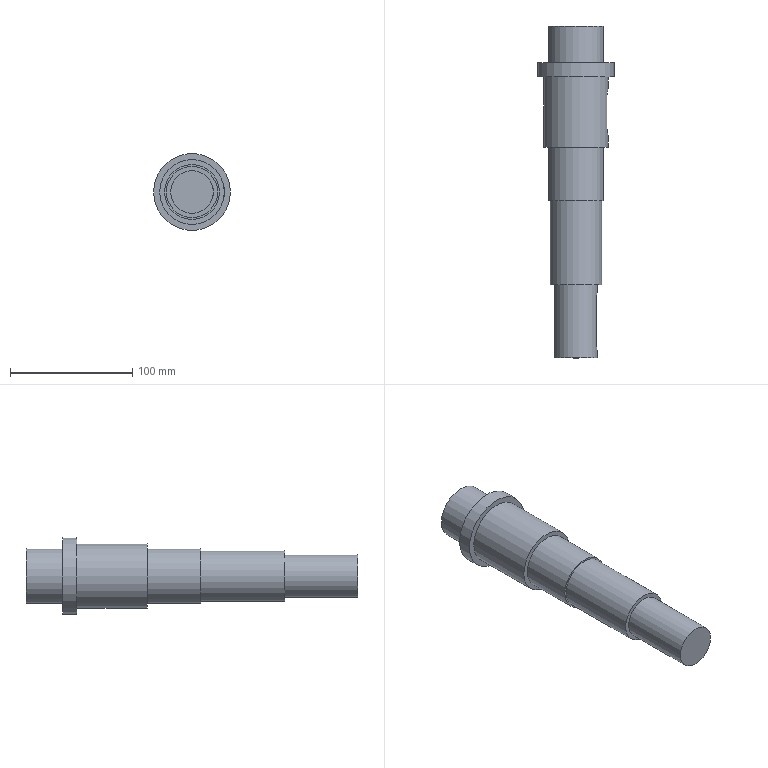Part | NX | features DATUM_CSYS 9, EXTRUDE 8, SKETCH 8, BLEND 2 | 1 solid | 23 faces | box 63 x 272 x 63 mm | volume 422770 mm3 | plane 13 | cylinder 10 | commonest cylinder face diameters 10 x2 16 x2 45 x2 35 x1 42 x1 53 x1
STEP:
#1=CARTESIAN_POINT('',(22.5,-30.,0.));
#2=VERTEX_POINT('',#1);
#3=CARTESIAN_POINT('',(0.,-30.,0.));
#4=DIRECTION('',(0.,-1.,0.));
#5=DIRECTION('',(1.,0.,0.));
#6=AXIS2_PLACEMENT_3D('',#3,#4,#5);
#7=CIRCLE('',#6,22.5);
#8=EDGE_CURVE('',#2,#2,#7,.T.);
#9=ORIENTED_EDGE('',*,*,#8,.F.);
#10=EDGE_LOOP('',(#9));
#11=FACE_BOUND('',#10,.T.);
#12=CARTESIAN_POINT('',(22.5,0.,0.));
#13=VERTEX_POINT('',#12);
#14=CARTESIAN_POINT('',(0.,0.,0.));
#15=DIRECTION('',(0.,-1.,0.));
#16=DIRECTION('',(1.,0.,0.));
#17=AXIS2_PLACEMENT_3D('',#14,#15,#16);
#18=CIRCLE('',#17,22.5);
#19=EDGE_CURVE('',#13,#13,#18,.T.);
#20=ORIENTED_EDGE('',*,*,#19,.T.);
#21=EDGE_LOOP('',(#20));
#22=FACE_BOUND('',#21,.T.);
#23=CARTESIAN_POINT('',(0.,-30.,0.));
#24=DIRECTION('',(0.,1.,0.));
#25=DIRECTION('',(0.,0.,1.));
#26=AXIS2_PLACEMENT_3D('',#23,#24,#25);
#27=CYLINDRICAL_SURFACE('',#26,22.5);
#28=ADVANCED_FACE('',(#11,#22),#27,.T.);
#29=ORIENTED_EDGE('',*,*,#19,.F.);
#30=EDGE_LOOP('',(#29));
#31=FACE_BOUND('',#30,.T.);
#32=CARTESIAN_POINT('',(0.,0.,0.));
#33=DIRECTION('',(0.,-1.,0.));
#34=DIRECTION('',(0.,0.,-1.));
#35=AXIS2_PLACEMENT_3D('',#32,#33,#34);
#36=PLANE('',#35);
#37=ADVANCED_FACE('',(#31),#36,.F.);
#38=CARTESIAN_POINT('',(31.5,-41.5,0.));
#39=VERTEX_POINT('',#38);
#40=CARTESIAN_POINT('',(0.,-41.5,0.));
#41=DIRECTION('',(0.,-1.,0.));
#42=DIRECTION('',(1.,0.,0.));
#43=AXIS2_PLACEMENT_3D('',#40,#41,#42);
#44=CIRCLE('',#43,31.5);
#45=EDGE_CURVE('',#39,#39,#44,.T.);
#46=ORIENTED_EDGE('',*,*,#45,.F.);
#47=EDGE_LOOP('',(#46));
#48=FACE_BOUND('',#47,.T.);
#49=CARTESIAN_POINT('',(31.5,-30.,0.));
#50=VERTEX_POINT('',#49);
#51=CARTESIAN_POINT('',(0.,-30.,0.));
#52=DIRECTION('',(0.,-1.,0.));
#53=DIRECTION('',(1.,0.,0.));
#54=AXIS2_PLACEMENT_3D('',#51,#52,#53);
#55=CIRCLE('',#54,31.5);
#56=EDGE_CURVE('',#50,#50,#55,.T.);
#57=ORIENTED_EDGE('',*,*,#56,.T.);
#58=EDGE_LOOP('',(#57));
#59=FACE_BOUND('',#58,.T.);
#60=CARTESIAN_POINT('',(0.,-41.5,0.));
#61=DIRECTION('',(0.,1.,0.));
#62=DIRECTION('',(0.,0.,1.));
#63=AXIS2_PLACEMENT_3D('',#60,#61,#62);
#64=CYLINDRICAL_SURFACE('',#63,31.5);
#65=ADVANCED_FACE('',(#48,#59),#64,.T.);
#66=CARTESIAN_POINT('',(26.5,-41.5,0.));
#67=VERTEX_POINT('',#66);
#68=CARTESIAN_POINT('',(0.,-41.5,0.));
#69=DIRECTION('',(0.,-1.,0.));
#70=DIRECTION('',(1.,0.,0.));
#71=AXIS2_PLACEMENT_3D('',#68,#69,#70);
#72=CIRCLE('',#71,26.5);
#73=EDGE_CURVE('',#67,#67,#72,.T.);
#74=ORIENTED_EDGE('',*,*,#73,.F.);
#75=EDGE_LOOP('',(#74));
#76=FACE_BOUND('',#75,.T.);
#77=ORIENTED_EDGE('',*,*,#45,.T.);
#78=EDGE_LOOP('',(#77));
#79=FACE_BOUND('',#78,.T.);
#80=CARTESIAN_POINT('',(0.,-41.5,0.));
#81=DIRECTION('',(0.,-1.,0.));
#82=DIRECTION('',(0.,0.,-1.));
#83=AXIS2_PLACEMENT_3D('',#80,#81,#82);
#84=PLANE('',#83);
#85=ADVANCED_FACE('',(#76,#79),#84,.T.);
#86=ORIENTED_EDGE('',*,*,#8,.T.);
#87=EDGE_LOOP('',(#86));
#88=FACE_BOUND('',#87,.T.);
#89=ORIENTED_EDGE('',*,*,#56,.F.);
#90=EDGE_LOOP('',(#89));
#91=FACE_BOUND('',#90,.T.);
#92=CARTESIAN_POINT('',(0.,-30.,0.));
#93=DIRECTION('',(0.,-1.,0.));
#94=DIRECTION('',(0.,0.,-1.));
#95=AXIS2_PLACEMENT_3D('',#92,#93,#94);
#96=PLANE('',#95);
#97=ADVANCED_FACE('',(#88,#91),#96,.F.);
#98=CARTESIAN_POINT('',(25.264,-82.5,-8.));
#99=VERTEX_POINT('',#98);
#100=CARTESIAN_POINT('',(25.264,-58.5,-8.));
#101=VERTEX_POINT('',#100);
#102=CARTESIAN_POINT('',(25.264,-99.5,-8.));
#103=DIRECTION('',(0.,1.,0.));
#104=VECTOR('',#103,1000.);
#105=LINE('',#102,#104);
#106=EDGE_CURVE('',#99,#101,#105,.T.);
#107=ORIENTED_EDGE('',*,*,#106,.F.);
#108=CARTESIAN_POINT('',(25.264,-82.5,8.));
#109=VERTEX_POINT('',#108);
#110=CARTESIAN_POINT('',(25.264,-82.5,-8.));
#111=CARTESIAN_POINT('',(25.264,-84.626,-8.));
#112=CARTESIAN_POINT('',(25.896,-88.747,-6.272));
#113=CARTESIAN_POINT('',(26.802,-91.375,0.001413));
#114=CARTESIAN_POINT('',(25.897,-88.752,6.267));
#115=CARTESIAN_POINT('',(25.264,-84.626,8.));
#116=CARTESIAN_POINT('',(25.264,-82.5,8.));
#117=B_SPLINE_CURVE_WITH_KNOTS('',3,(#110,#111,#112,#113,#114,#115,#116),.UNSPECIFIED.,.F.,.F.,(4,1,1,1,4),(-0.01257,-0.006285,0.000000113,0.006286,0.01257),.UNSPECIFIED.);
#118=EDGE_CURVE('',#99,#109,#117,.T.);
#119=ORIENTED_EDGE('',*,*,#118,.T.);
#120=CARTESIAN_POINT('',(25.264,-58.5,8.));
#121=VERTEX_POINT('',#120);
#122=CARTESIAN_POINT('',(25.264,-99.5,8.));
#123=DIRECTION('',(0.,1.,0.));
#124=VECTOR('',#123,1000.);
#125=LINE('',#122,#124);
#126=EDGE_CURVE('',#109,#121,#125,.T.);
#127=ORIENTED_EDGE('',*,*,#126,.T.);
#128=CARTESIAN_POINT('',(25.264,-58.5,8.));
#129=CARTESIAN_POINT('',(25.264,-56.374,8.));
#130=CARTESIAN_POINT('',(25.896,-52.253,6.272));
#131=CARTESIAN_POINT('',(26.802,-49.625,-0.001413));
#132=CARTESIAN_POINT('',(25.897,-52.248,-6.267));
#133=CARTESIAN_POINT('',(25.264,-56.374,-8.));
#134=CARTESIAN_POINT('',(25.264,-58.5,-8.));
#135=B_SPLINE_CURVE_WITH_KNOTS('',3,(#128,#129,#130,#131,#132,#133,#134),.UNSPECIFIED.,.F.,.F.,(4,1,1,1,4),(0.,0.006286,0.01257,0.01886,0.02514),.UNSPECIFIED.);
#136=EDGE_CURVE('',#121,#101,#135,.T.);
#137=ORIENTED_EDGE('',*,*,#136,.T.);
#138=EDGE_LOOP('',(#107,#119,#127,#137));
#139=FACE_BOUND('',#138,.T.);
#140=CARTESIAN_POINT('',(26.5,-99.5,0.));
#141=VERTEX_POINT('',#140);
#142=CARTESIAN_POINT('',(0.,-99.5,0.));
#143=DIRECTION('',(0.,-1.,0.));
#144=DIRECTION('',(1.,0.,0.));
#145=AXIS2_PLACEMENT_3D('',#142,#143,#144);
#146=CIRCLE('',#145,26.5);
#147=EDGE_CURVE('',#141,#141,#146,.T.);
#148=ORIENTED_EDGE('',*,*,#147,.F.);
#149=EDGE_LOOP('',(#148));
#150=FACE_BOUND('',#149,.T.);
#151=ORIENTED_EDGE('',*,*,#73,.T.);
#152=EDGE_LOOP('',(#151));
#153=FACE_BOUND('',#152,.T.);
#154=CARTESIAN_POINT('',(0.,-99.5,0.));
#155=DIRECTION('',(0.,1.,0.));
#156=DIRECTION('',(0.,0.,1.));
#157=AXIS2_PLACEMENT_3D('',#154,#155,#156);
#158=CYLINDRICAL_SURFACE('',#157,26.5);
#159=ADVANCED_FACE('',(#139,#150,#153),#158,.T.);
#160=CARTESIAN_POINT('',(22.5,-99.5,0.));
#161=VERTEX_POINT('',#160);
#162=CARTESIAN_POINT('',(0.,-99.5,0.));
#163=DIRECTION('',(0.,-1.,0.));
#164=DIRECTION('',(1.,0.,0.));
#165=AXIS2_PLACEMENT_3D('',#162,#163,#164);
#166=CIRCLE('',#165,22.5);
#167=EDGE_CURVE('',#161,#161,#166,.T.);
#168=ORIENTED_EDGE('',*,*,#167,.F.);
#169=EDGE_LOOP('',(#168));
#170=FACE_BOUND('',#169,.T.);
#171=ORIENTED_EDGE('',*,*,#147,.T.);
#172=EDGE_LOOP('',(#171));
#173=FACE_BOUND('',#172,.T.);
#174=CARTESIAN_POINT('',(0.,-99.5,0.));
#175=DIRECTION('',(0.,-1.,0.));
#176=DIRECTION('',(0.,0.,-1.));
#177=AXIS2_PLACEMENT_3D('',#174,#175,#176);
#178=PLANE('',#177);
#179=ADVANCED_FACE('',(#170,#173),#178,.T.);
#180=CARTESIAN_POINT('',(22.5,-143.,0.));
#181=VERTEX_POINT('',#180);
#182=CARTESIAN_POINT('',(0.,-143.,0.));
#183=DIRECTION('',(0.,-1.,0.));
#184=DIRECTION('',(1.,0.,0.));
#185=AXIS2_PLACEMENT_3D('',#182,#183,#184);
#186=CIRCLE('',#185,22.5);
#187=EDGE_CURVE('',#181,#181,#186,.T.);
#188=ORIENTED_EDGE('',*,*,#187,.F.);
#189=EDGE_LOOP('',(#188));
#190=FACE_BOUND('',#189,.T.);
#191=ORIENTED_EDGE('',*,*,#167,.T.);
#192=EDGE_LOOP('',(#191));
#193=FACE_BOUND('',#192,.T.);
#194=CARTESIAN_POINT('',(0.,-143.,0.));
#195=DIRECTION('',(0.,1.,0.));
#196=DIRECTION('',(0.,0.,1.));
#197=AXIS2_PLACEMENT_3D('',#194,#195,#196);
#198=CYLINDRICAL_SURFACE('',#197,22.5);
#199=ADVANCED_FACE('',(#190,#193),#198,.T.);
#200=CARTESIAN_POINT('',(21.,-143.,0.));
#201=VERTEX_POINT('',#200);
#202=CARTESIAN_POINT('',(0.,-143.,0.));
#203=DIRECTION('',(0.,-1.,0.));
#204=DIRECTION('',(1.,0.,0.));
#205=AXIS2_PLACEMENT_3D('',#202,#203,#204);
#206=CIRCLE('',#205,21.);
#207=EDGE_CURVE('',#201,#201,#206,.T.);
#208=ORIENTED_EDGE('',*,*,#207,.F.);
#209=EDGE_LOOP('',(#208));
#210=FACE_BOUND('',#209,.T.);
#211=ORIENTED_EDGE('',*,*,#187,.T.);
#212=EDGE_LOOP('',(#211));
#213=FACE_BOUND('',#212,.T.);
#214=CARTESIAN_POINT('',(0.,-143.,0.));
#215=DIRECTION('',(0.,-1.,0.));
#216=DIRECTION('',(0.,0.,-1.));
#217=AXIS2_PLACEMENT_3D('',#214,#215,#216);
#218=PLANE('',#217);
#219=ADVANCED_FACE('',(#210,#213),#218,.T.);
#220=CARTESIAN_POINT('',(21.,-212.,0.));
#221=VERTEX_POINT('',#220);
#222=CARTESIAN_POINT('',(0.,-212.,0.));
#223=DIRECTION('',(0.,-1.,0.));
#224=DIRECTION('',(1.,0.,0.));
#225=AXIS2_PLACEMENT_3D('',#222,#223,#224);
#226=CIRCLE('',#225,21.);
#227=EDGE_CURVE('',#221,#221,#226,.T.);
#228=ORIENTED_EDGE('',*,*,#227,.F.);
#229=EDGE_LOOP('',(#228));
#230=FACE_BOUND('',#229,.T.);
#231=ORIENTED_EDGE('',*,*,#207,.T.);
#232=EDGE_LOOP('',(#231));
#233=FACE_BOUND('',#232,.T.);
#234=CARTESIAN_POINT('',(0.,-212.,0.));
#235=DIRECTION('',(0.,1.,0.));
#236=DIRECTION('',(0.,0.,1.));
#237=AXIS2_PLACEMENT_3D('',#234,#235,#236);
#238=CYLINDRICAL_SURFACE('',#237,21.);
#239=ADVANCED_FACE('',(#230,#233),#238,.T.);
#240=CARTESIAN_POINT('',(17.5,-212.,0.));
#241=VERTEX_POINT('',#240);
#242=CARTESIAN_POINT('',(0.,-212.,0.));
#243=DIRECTION('',(0.,-1.,0.));
#244=DIRECTION('',(1.,0.,0.));
#245=AXIS2_PLACEMENT_3D('',#242,#243,#244);
#246=CIRCLE('',#245,17.5);
#247=EDGE_CURVE('',#241,#241,#246,.T.);
#248=ORIENTED_EDGE('',*,*,#247,.F.);
#249=EDGE_LOOP('',(#248));
#250=FACE_BOUND('',#249,.T.);
#251=ORIENTED_EDGE('',*,*,#227,.T.);
#252=EDGE_LOOP('',(#251));
#253=FACE_BOUND('',#252,.T.);
#254=CARTESIAN_POINT('',(0.,-212.,0.));
#255=DIRECTION('',(0.,-1.,0.));
#256=DIRECTION('',(0.,0.,-1.));
#257=AXIS2_PLACEMENT_3D('',#254,#255,#256);
#258=PLANE('',#257);
#259=ADVANCED_FACE('',(#250,#253),#258,.T.);
#260=CARTESIAN_POINT('',(16.771,-262.,-5.));
#261=VERTEX_POINT('',#260);
#262=CARTESIAN_POINT('',(16.771,-222.,-5.));
#263=VERTEX_POINT('',#262);
#264=CARTESIAN_POINT('',(16.771,-272.,-5.));
#265=DIRECTION('',(0.,1.,0.));
#266=VECTOR('',#265,1000.);
#267=LINE('',#264,#266);
#268=EDGE_CURVE('',#261,#263,#267,.T.);
#269=ORIENTED_EDGE('',*,*,#268,.F.);
#270=CARTESIAN_POINT('',(16.771,-262.,5.));
#271=VERTEX_POINT('',#270);
#272=CARTESIAN_POINT('',(16.771,-262.,-5.));
#273=CARTESIAN_POINT('',(16.771,-263.328,-5.));
#274=CARTESIAN_POINT('',(17.143,-265.905,-3.92));
#275=CARTESIAN_POINT('',(17.679,-267.547,0.0009525));
#276=CARTESIAN_POINT('',(17.143,-265.908,3.917));
#277=CARTESIAN_POINT('',(16.771,-263.328,5.));
#278=CARTESIAN_POINT('',(16.771,-262.,5.));
#279=B_SPLINE_CURVE_WITH_KNOTS('',3,(#272,#273,#274,#275,#276,#277,#278),.UNSPECIFIED.,.F.,.F.,(4,1,1,1,4),(-0.007852,-0.003926,0.000000084,0.003926,0.007852),.UNSPECIFIED.);
#280=EDGE_CURVE('',#261,#271,#279,.T.);
#281=ORIENTED_EDGE('',*,*,#280,.T.);
#282=CARTESIAN_POINT('',(16.771,-222.,5.));
#283=VERTEX_POINT('',#282);
#284=CARTESIAN_POINT('',(16.771,-272.,5.));
#285=DIRECTION('',(0.,1.,0.));
#286=VECTOR('',#285,1000.);
#287=LINE('',#284,#286);
#288=EDGE_CURVE('',#271,#283,#287,.T.);
#289=ORIENTED_EDGE('',*,*,#288,.T.);
#290=CARTESIAN_POINT('',(16.771,-222.,5.));
#291=CARTESIAN_POINT('',(16.771,-220.672,5.));
#292=CARTESIAN_POINT('',(17.143,-218.095,3.92));
#293=CARTESIAN_POINT('',(17.679,-216.453,-0.0009525));
#294=CARTESIAN_POINT('',(17.143,-218.092,-3.917));
#295=CARTESIAN_POINT('',(16.771,-220.672,-5.));
#296=CARTESIAN_POINT('',(16.771,-222.,-5.));
#297=B_SPLINE_CURVE_WITH_KNOTS('',3,(#290,#291,#292,#293,#294,#295,#296),.UNSPECIFIED.,.F.,.F.,(4,1,1,1,4),(0.,0.003926,0.007852,0.01178,0.0157),.UNSPECIFIED.);
#298=EDGE_CURVE('',#283,#263,#297,.T.);
#299=ORIENTED_EDGE('',*,*,#298,.T.);
#300=EDGE_LOOP('',(#269,#281,#289,#299));
#301=FACE_BOUND('',#300,.T.);
#302=CARTESIAN_POINT('',(17.5,-272.,0.));
#303=VERTEX_POINT('',#302);
#304=CARTESIAN_POINT('',(0.,-272.,0.));
#305=DIRECTION('',(0.,-1.,0.));
#306=DIRECTION('',(1.,0.,0.));
#307=AXIS2_PLACEMENT_3D('',#304,#305,#306);
#308=CIRCLE('',#307,17.5);
#309=EDGE_CURVE('',#303,#303,#308,.T.);
#310=ORIENTED_EDGE('',*,*,#309,.F.);
#311=EDGE_LOOP('',(#310));
#312=FACE_BOUND('',#311,.T.);
#313=ORIENTED_EDGE('',*,*,#247,.T.);
#314=EDGE_LOOP('',(#313));
#315=FACE_BOUND('',#314,.T.);
#316=CARTESIAN_POINT('',(0.,-272.,0.));
#317=DIRECTION('',(0.,1.,0.));
#318=DIRECTION('',(0.,0.,1.));
#319=AXIS2_PLACEMENT_3D('',#316,#317,#318);
#320=CYLINDRICAL_SURFACE('',#319,17.5);
#321=ADVANCED_FACE('',(#301,#312,#315),#320,.T.);
#322=ORIENTED_EDGE('',*,*,#309,.T.);
#323=EDGE_LOOP('',(#322));
#324=FACE_BOUND('',#323,.T.);
#325=CARTESIAN_POINT('',(0.,-272.,0.));
#326=DIRECTION('',(0.,-1.,0.));
#327=DIRECTION('',(0.,0.,-1.));
#328=AXIS2_PLACEMENT_3D('',#325,#326,#327);
#329=PLANE('',#328);
#330=ADVANCED_FACE('',(#324),#329,.T.);
#331=ORIENTED_EDGE('',*,*,#288,.F.);
#332=CARTESIAN_POINT('',(9.,-262.,5.));
#333=VERTEX_POINT('',#332);
#334=CARTESIAN_POINT('',(0.,-262.,5.));
#335=DIRECTION('',(-1.,0.,0.));
#336=VECTOR('',#335,1000.);
#337=LINE('',#334,#336);
#338=EDGE_CURVE('',#271,#333,#337,.T.);
#339=ORIENTED_EDGE('',*,*,#338,.T.);
#340=CARTESIAN_POINT('',(9.,-222.,5.));
#341=VERTEX_POINT('',#340);
#342=CARTESIAN_POINT('',(9.,-217.,5.));
#343=DIRECTION('',(0.,-1.,0.));
#344=VECTOR('',#343,1000.);
#345=LINE('',#342,#344);
#346=EDGE_CURVE('',#333,#341,#345,.F.);
#347=ORIENTED_EDGE('',*,*,#346,.T.);
#348=CARTESIAN_POINT('',(0.,-222.,5.));
#349=DIRECTION('',(1.,0.,0.));
#350=VECTOR('',#349,1000.);
#351=LINE('',#348,#350);
#352=EDGE_CURVE('',#341,#283,#351,.T.);
#353=ORIENTED_EDGE('',*,*,#352,.T.);
#354=EDGE_LOOP('',(#331,#339,#347,#353));
#355=FACE_BOUND('',#354,.T.);
#356=CARTESIAN_POINT('',(0.,0.,5.));
#357=DIRECTION('',(0.,0.,1.));
#358=DIRECTION('',(1.,0.,0.));
#359=AXIS2_PLACEMENT_3D('',#356,#357,#358);
#360=PLANE('',#359);
#361=ADVANCED_FACE('',(#355),#360,.F.);
#362=CARTESIAN_POINT('',(9.,-262.,-5.));
#363=VERTEX_POINT('',#362);
#364=CARTESIAN_POINT('',(9.,-222.,-5.));
#365=VERTEX_POINT('',#364);
#366=CARTESIAN_POINT('',(9.,-217.,-5.));
#367=DIRECTION('',(0.,-1.,0.));
#368=VECTOR('',#367,1000.);
#369=LINE('',#366,#368);
#370=EDGE_CURVE('',#363,#365,#369,.F.);
#371=ORIENTED_EDGE('',*,*,#370,.F.);
#372=CARTESIAN_POINT('',(16.771,-262.,-5.));
#373=DIRECTION('',(-1.,0.,0.));
#374=VECTOR('',#373,1000.);
#375=LINE('',#372,#374);
#376=EDGE_CURVE('',#363,#261,#375,.F.);
#377=ORIENTED_EDGE('',*,*,#376,.T.);
#378=ORIENTED_EDGE('',*,*,#268,.T.);
#379=CARTESIAN_POINT('',(9.,-222.,-5.));
#380=DIRECTION('',(1.,0.,0.));
#381=VECTOR('',#380,1000.);
#382=LINE('',#379,#381);
#383=EDGE_CURVE('',#263,#365,#382,.F.);
#384=ORIENTED_EDGE('',*,*,#383,.T.);
#385=EDGE_LOOP('',(#371,#377,#378,#384));
#386=FACE_BOUND('',#385,.T.);
#387=CARTESIAN_POINT('',(0.,0.,-5.));
#388=DIRECTION('',(0.,0.,1.));
#389=DIRECTION('',(1.,0.,0.));
#390=AXIS2_PLACEMENT_3D('',#387,#388,#389);
#391=PLANE('',#390);
#392=ADVANCED_FACE('',(#386),#391,.T.);
#393=ORIENTED_EDGE('',*,*,#346,.F.);
#394=CARTESIAN_POINT('',(9.,-262.,0.));
#395=DIRECTION('',(1.,0.,0.));
#396=DIRECTION('',(0.,1.,0.));
#397=AXIS2_PLACEMENT_3D('',#394,#395,#396);
#398=CIRCLE('',#397,5.);
#399=EDGE_CURVE('',#333,#363,#398,.T.);
#400=ORIENTED_EDGE('',*,*,#399,.T.);
#401=ORIENTED_EDGE('',*,*,#370,.T.);
#402=CARTESIAN_POINT('',(9.,-222.,0.));
#403=DIRECTION('',(1.,0.,0.));
#404=DIRECTION('',(0.,1.,0.));
#405=AXIS2_PLACEMENT_3D('',#402,#403,#404);
#406=CIRCLE('',#405,5.);
#407=EDGE_CURVE('',#365,#341,#406,.T.);
#408=ORIENTED_EDGE('',*,*,#407,.T.);
#409=EDGE_LOOP('',(#393,#400,#401,#408));
#410=FACE_BOUND('',#409,.T.);
#411=CARTESIAN_POINT('',(9.,-217.,5.));
#412=DIRECTION('',(1.,0.,0.));
#413=DIRECTION('',(0.,1.,0.));
#414=AXIS2_PLACEMENT_3D('',#411,#412,#413);
#415=PLANE('',#414);
#416=ADVANCED_FACE('',(#410),#415,.T.);
#417=ORIENTED_EDGE('',*,*,#399,.F.);
#418=ORIENTED_EDGE('',*,*,#338,.F.);
#419=ORIENTED_EDGE('',*,*,#280,.F.);
#420=ORIENTED_EDGE('',*,*,#376,.F.);
#421=EDGE_LOOP('',(#417,#418,#419,#420));
#422=FACE_BOUND('',#421,.T.);
#423=CARTESIAN_POINT('',(9.,-262.,0.));
#424=DIRECTION('',(1.,0.,0.));
#425=DIRECTION('',(0.,0.,-1.));
#426=AXIS2_PLACEMENT_3D('',#423,#424,#425);
#427=CYLINDRICAL_SURFACE('',#426,5.);
#428=ADVANCED_FACE('',(#422),#427,.F.);
#429=ORIENTED_EDGE('',*,*,#383,.F.);
#430=ORIENTED_EDGE('',*,*,#298,.F.);
#431=ORIENTED_EDGE('',*,*,#352,.F.);
#432=ORIENTED_EDGE('',*,*,#407,.F.);
#433=EDGE_LOOP('',(#429,#430,#431,#432));
#434=FACE_BOUND('',#433,.T.);
#435=CARTESIAN_POINT('',(24.,-222.,0.));
#436=DIRECTION('',(-1.,0.,0.));
#437=DIRECTION('',(0.,0.,1.));
#438=AXIS2_PLACEMENT_3D('',#435,#436,#437);
#439=CYLINDRICAL_SURFACE('',#438,5.);
#440=ADVANCED_FACE('',(#434),#439,.F.);
#441=ORIENTED_EDGE('',*,*,#126,.F.);
#442=CARTESIAN_POINT('',(13.649,-82.5,8.));
#443=VERTEX_POINT('',#442);
#444=CARTESIAN_POINT('',(0.,-82.5,8.));
#445=DIRECTION('',(-1.,0.,0.));
#446=VECTOR('',#445,1000.);
#447=LINE('',#444,#446);
#448=EDGE_CURVE('',#109,#443,#447,.T.);
#449=ORIENTED_EDGE('',*,*,#448,.T.);
#450=CARTESIAN_POINT('',(13.649,-58.5,8.));
#451=VERTEX_POINT('',#450);
#452=CARTESIAN_POINT('',(13.649,-50.5,8.));
#453=DIRECTION('',(0.,-1.,0.));
#454=VECTOR('',#453,1000.);
#455=LINE('',#452,#454);
#456=EDGE_CURVE('',#443,#451,#455,.F.);
#457=ORIENTED_EDGE('',*,*,#456,.T.);
#458=CARTESIAN_POINT('',(0.,-58.5,8.));
#459=DIRECTION('',(1.,0.,0.));
#460=VECTOR('',#459,1000.);
#461=LINE('',#458,#460);
#462=EDGE_CURVE('',#451,#121,#461,.T.);
#463=ORIENTED_EDGE('',*,*,#462,.T.);
#464=EDGE_LOOP('',(#441,#449,#457,#463));
#465=FACE_BOUND('',#464,.T.);
#466=CARTESIAN_POINT('',(0.,0.,8.));
#467=DIRECTION('',(0.,0.,1.));
#468=DIRECTION('',(1.,0.,0.));
#469=AXIS2_PLACEMENT_3D('',#466,#467,#468);
#470=PLANE('',#469);
#471=ADVANCED_FACE('',(#465),#470,.F.);
#472=ORIENTED_EDGE('',*,*,#106,.T.);
#473=CARTESIAN_POINT('',(13.649,-58.5,-8.));
#474=VERTEX_POINT('',#473);
#475=CARTESIAN_POINT('',(13.649,-58.5,-8.));
#476=DIRECTION('',(1.,0.,0.));
#477=VECTOR('',#476,1000.);
#478=LINE('',#475,#477);
#479=EDGE_CURVE('',#101,#474,#478,.F.);
#480=ORIENTED_EDGE('',*,*,#479,.T.);
#481=CARTESIAN_POINT('',(13.649,-82.5,-8.));
#482=VERTEX_POINT('',#481);
#483=CARTESIAN_POINT('',(13.649,-50.5,-8.));
#484=DIRECTION('',(0.,-1.,0.));
#485=VECTOR('',#484,1000.);
#486=LINE('',#483,#485);
#487=EDGE_CURVE('',#482,#474,#486,.F.);
#488=ORIENTED_EDGE('',*,*,#487,.F.);
#489=CARTESIAN_POINT('',(25.264,-82.5,-8.));
#490=DIRECTION('',(-1.,0.,0.));
#491=VECTOR('',#490,1000.);
#492=LINE('',#489,#491);
#493=EDGE_CURVE('',#482,#99,#492,.F.);
#494=ORIENTED_EDGE('',*,*,#493,.T.);
#495=EDGE_LOOP('',(#472,#480,#488,#494));
#496=FACE_BOUND('',#495,.T.);
#497=CARTESIAN_POINT('',(0.,0.,-8.));
#498=DIRECTION('',(0.,0.,1.));
#499=DIRECTION('',(1.,0.,0.));
#500=AXIS2_PLACEMENT_3D('',#497,#498,#499);
#501=PLANE('',#500);
#502=ADVANCED_FACE('',(#496),#501,.T.);
#503=CARTESIAN_POINT('',(13.649,-58.5,0.));
#504=DIRECTION('',(1.,0.,0.));
#505=DIRECTION('',(0.,1.,0.));
#506=AXIS2_PLACEMENT_3D('',#503,#504,#505);
#507=CIRCLE('',#506,8.);
#508=EDGE_CURVE('',#474,#451,#507,.T.);
#509=ORIENTED_EDGE('',*,*,#508,.T.);
#510=ORIENTED_EDGE('',*,*,#456,.F.);
#511=CARTESIAN_POINT('',(13.649,-82.5,0.));
#512=DIRECTION('',(1.,0.,0.));
#513=DIRECTION('',(0.,1.,0.));
#514=AXIS2_PLACEMENT_3D('',#511,#512,#513);
#515=CIRCLE('',#514,8.);
#516=EDGE_CURVE('',#443,#482,#515,.T.);
#517=ORIENTED_EDGE('',*,*,#516,.T.);
#518=ORIENTED_EDGE('',*,*,#487,.T.);
#519=EDGE_LOOP('',(#509,#510,#517,#518));
#520=FACE_BOUND('',#519,.T.);
#521=CARTESIAN_POINT('',(13.649,-50.5,8.));
#522=DIRECTION('',(1.,0.,0.));
#523=DIRECTION('',(0.,1.,0.));
#524=AXIS2_PLACEMENT_3D('',#521,#522,#523);
#525=PLANE('',#524);
#526=ADVANCED_FACE('',(#520),#525,.T.);
#527=ORIENTED_EDGE('',*,*,#516,.F.);
#528=ORIENTED_EDGE('',*,*,#448,.F.);
#529=ORIENTED_EDGE('',*,*,#118,.F.);
#530=ORIENTED_EDGE('',*,*,#493,.F.);
#531=EDGE_LOOP('',(#527,#528,#529,#530));
#532=FACE_BOUND('',#531,.T.);
#533=CARTESIAN_POINT('',(13.649,-82.5,0.));
#534=DIRECTION('',(1.,0.,0.));
#535=DIRECTION('',(0.,1.,0.));
#536=AXIS2_PLACEMENT_3D('',#533,#534,#535);
#537=CYLINDRICAL_SURFACE('',#536,8.);
#538=ADVANCED_FACE('',(#532),#537,.F.);
#539=ORIENTED_EDGE('',*,*,#479,.F.);
#540=ORIENTED_EDGE('',*,*,#136,.F.);
#541=ORIENTED_EDGE('',*,*,#462,.F.);
#542=ORIENTED_EDGE('',*,*,#508,.F.);
#543=EDGE_LOOP('',(#539,#540,#541,#542));
#544=FACE_BOUND('',#543,.T.);
#545=CARTESIAN_POINT('',(37.,-58.5,0.));
#546=DIRECTION('',(-1.,0.,0.));
#547=DIRECTION('',(0.,0.,1.));
#548=AXIS2_PLACEMENT_3D('',#545,#546,#547);
#549=CYLINDRICAL_SURFACE('',#548,8.);
#550=ADVANCED_FACE('',(#544),#549,.F.);
#551=CLOSED_SHELL('',(#28,#37,#65,#85,#97,#159,#179,#199,#219,#239,#259,#321,#330,#361,#392,#416,#428,#440,#471,#502,#526,#538,#550));
#552=MANIFOLD_SOLID_BREP('',#551);
#553=(LENGTH_UNIT()NAMED_UNIT(*)SI_UNIT(.MILLI.,.METRE.));
#554=UNCERTAINTY_MEASURE_WITH_UNIT(LENGTH_MEASURE(0.0508),#553,'','');
#555=(NAMED_UNIT(*)PLANE_ANGLE_UNIT()SI_UNIT($,.RADIAN.));
#556=(NAMED_UNIT(*)SI_UNIT($,.STERADIAN.)SOLID_ANGLE_UNIT());
#557=(GEOMETRIC_REPRESENTATION_CONTEXT(3)GLOBAL_UNCERTAINTY_ASSIGNED_CONTEXT((#554))GLOBAL_UNIT_ASSIGNED_CONTEXT((#553,#555,#556))REPRESENTATION_CONTEXT('',''));
#558=ADVANCED_BREP_SHAPE_REPRESENTATION('',(#552),#557);